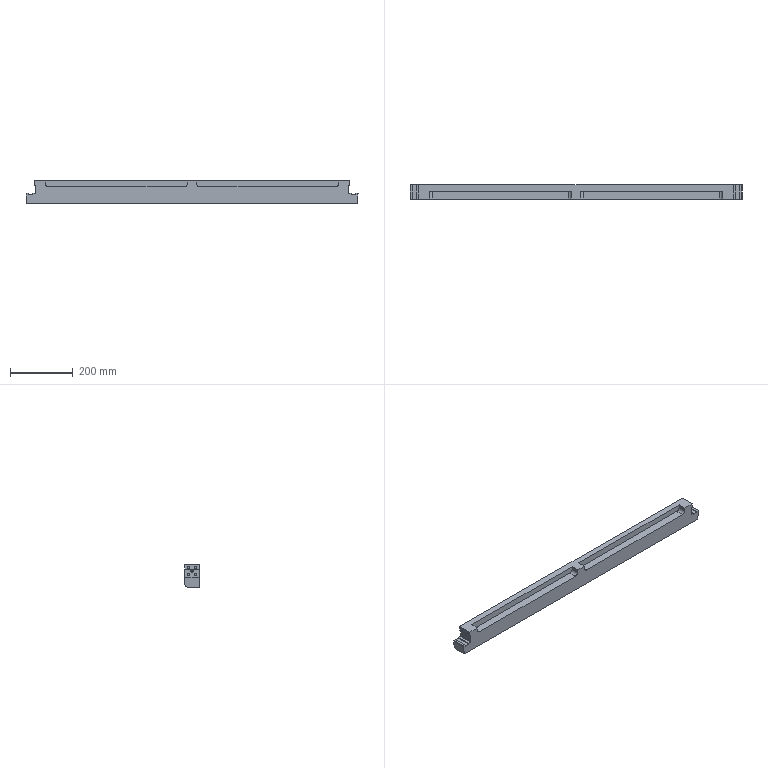NC program | NX | posted with a generic post | part box 1056 x 45 x 72.5 mm
Whole program:
N10 G17 G21 G94 G90
(ZLEVEL_PROFILE_2 , TOOL : D12)
N12 T20 M6
N14 G54
N16 G17 G0 G90 X-200.083 Y18.15 B0. C0. S7500 M3
N18 G43 Z30. H20
N20 Z1.5
N22 G94 G1 X-266. Z-1.955 F1001.
N24 X-482. F3000.
N26 G3 X-486.4 Y13.75 R4.4
N28 X-482. Y9.35 R4.4
N30 G1 X-50.
N32 G3 X-45.6 Y13.75 R4.4
N34 X-50. Y18.15 R4.4
N36 G1 X-266.
N38 X-377.976 Z-3.909
N40 X-482.
N42 G3 X-486.4 Y13.75 R4.4
N44 X-482. Y9.35 R4.4
N46 G1 X-50.
N48 G3 X-45.6 Y13.75 R4.4
N50 X-50. Y18.15 R4.4
N52 G1 X-266.
N54 X-377.976 Z-5.864
N56 X-482.
N58 G3 X-486.4 Y13.75 R4.4
N60 X-482. Y9.35 R4.4
N62 G1 X-50.
N64 G3 X-45.6 Y13.75 R4.4
N66 X-50. Y18.15 R4.4
N68 G1 X-266.
N70 X-377.976 Z-7.818
N72 X-482.
N74 G3 X-486.4 Y13.75 R4.4
N76 X-482. Y9.35 R4.4
N78 G1 X-50.
N80 G3 X-45.6 Y13.75 R4.4
N82 X-50. Y18.15 R4.4
N84 G1 X-266.
N86 X-377.976 Z-9.773
N88 X-482.
N90 G3 X-486.4 Y13.75 R4.4
N92 X-482. Y9.35 R4.4
N94 G1 X-50.
N96 G3 X-45.6 Y13.75 R4.4
N98 X-50. Y18.15 R4.4
N100 G1 X-266.
N102 X-377.976 Z-11.727
N104 X-482.
N106 G3 X-486.4 Y13.75 R4.4
N108 X-482. Y9.35 R4.4
N110 G1 X-50.
N112 G3 X-45.6 Y13.75 R4.4
N114 X-50. Y18.15 R4.4
N116 G1 X-266.
N118 X-377.976 Z-13.682
N120 X-482.
N122 G3 X-486.4 Y13.75 R4.4
N124 X-482. Y9.35 R4.4
N126 G1 X-50.
N128 G3 X-45.6 Y13.75 R4.4
N130 X-50. Y18.15 R4.4
N132 G1 X-266.
N134 X-377.976 Z-15.636
N136 X-482.
N138 G3 X-486.4 Y13.75 R4.4
N140 X-482. Y9.35 R4.4
N142 G1 X-50.
N144 G3 X-45.6 Y13.75 R4.4
N146 X-50. Y18.15 R4.4
N148 G1 X-266.
N150 X-377.976 Z-17.591
N152 X-482.
N154 G3 X-486.4 Y13.75 R4.4
N156 X-482. Y9.35 R4.4
N158 G1 X-50.
N160 G3 X-45.6 Y13.75 R4.4
N162 X-50. Y18.15 R4.4
N164 G1 X-266.
N166 X-377.976 Z-19.545
N168 X-482.
N170 G3 X-486.4 Y13.75 R4.4
N172 X-482. Y9.35 R4.4
N174 G1 X-50.
N176 G3 X-45.6 Y13.75 R4.4
N178 X-50. Y18.15 R4.4
N180 G1 X-266.
N182 X-377.976 Z-21.5
N184 X-482.
N186 G3 X-486.4 Y13.75 R4.4
N188 X-482. Y9.35 R4.4
N190 G1 X-50.
N192 G3 X-45.6 Y13.75 R4.4
N194 X-50. Y18.15 R4.4
N196 G1 X-377.976
N198 G3 X-379.015 Y17.55 R1.2
N200 G1 X-379.361 Y16.95
N202 Z-20.3
N204 G0 Z30.
N206 X331.917 Y18.15
N208 Z1.5
N210 G1 X266. Z-1.955 F1001.
N212 X50. F3000.
N214 G3 X45.6 Y13.75 R4.4
N216 X50. Y9.35 R4.4
N218 G1 X482.
N220 G3 X486.4 Y13.75 R4.4
N222 X482. Y18.15 R4.4
N224 G1 X266.
N226 X154.024 Z-3.909
N228 X50.
N230 G3 X45.6 Y13.75 R4.4
N232 X50. Y9.35 R4.4
N234 G1 X482.
N236 G3 X486.4 Y13.75 R4.4
N238 X482. Y18.15 R4.4
N240 G1 X266.
N242 X154.024 Z-5.864
N244 X50.
N246 G3 X45.6 Y13.75 R4.4
N248 X50. Y9.35 R4.4
N250 G1 X482.
N252 G3 X486.4 Y13.75 R4.4
N254 X482. Y18.15 R4.4
N256 G1 X266.
N258 X154.024 Z-7.818
N260 X50.
N262 G3 X45.6 Y13.75 R4.4
N264 X50. Y9.35 R4.4
N266 G1 X482.
N268 G3 X486.4 Y13.75 R4.4
N270 X482. Y18.15 R4.4
N272 G1 X266.
N274 X154.024 Z-9.773
N276 X50.
N278 G3 X45.6 Y13.75 R4.4
N280 X50. Y9.35 R4.4
N282 G1 X482.
N284 G3 X486.4 Y13.75 R4.4
N286 X482. Y18.15 R4.4
N288 G1 X266.
N290 X154.024 Z-11.727
N292 X50.
N294 G3 X45.6 Y13.75 R4.4
N296 X50. Y9.35 R4.4
N298 G1 X482.
N300 G3 X486.4 Y13.75 R4.4
N302 X482. Y18.15 R4.4
N304 G1 X266.
N306 X154.024 Z-13.682
N308 X50.
N310 G3 X45.6 Y13.75 R4.4
N312 X50. Y9.35 R4.4
N314 G1 X482.
N316 G3 X486.4 Y13.75 R4.4
N318 X482. Y18.15 R4.4
N320 G1 X266.
N322 X154.024 Z-15.636
N324 X50.
N326 G3 X45.6 Y13.75 R4.4
N328 X50. Y9.35 R4.4
N330 G1 X482.
N332 G3 X486.4 Y13.75 R4.4
N334 X482. Y18.15 R4.4
N336 G1 X266.
N338 X154.024 Z-17.591
N340 X50.
N342 G3 X45.6 Y13.75 R4.4
N344 X50. Y9.35 R4.4
N346 G1 X482.
N348 G3 X486.4 Y13.75 R4.4
N350 X482. Y18.15 R4.4
N352 G1 X266.
N354 X154.024 Z-19.545
N356 X50.
N358 G3 X45.6 Y13.75 R4.4
N360 X50. Y9.35 R4.4
N362 G1 X482.
N364 G3 X486.4 Y13.75 R4.4
N366 X482. Y18.15 R4.4
N368 G1 X266.
N370 X154.024 Z-21.5
N372 X50.
N374 G3 X45.6 Y13.75 R4.4
N376 X50. Y9.35 R4.4
N378 G1 X482.
N380 G3 X486.4 Y13.75 R4.4
N382 X482. Y18.15 R4.4
N384 G1 X154.024
N386 G3 X152.985 Y17.55 R1.2
N388 G1 X152.639 Y16.95
N390 Z-20.3
N392 G0 Z30.
(11 , TOOL : D12)
N394 X-49.459 Y15.779 S6500
N396 Z-20.5
N398 G1 Z-21.5 F1000.
N400 X-48.961 Y17.65
N402 G3 X-50. Y18.25 R1.2
N404 G1 X-482.
N406 G3 X-486.5 Y13.75 R4.5
N408 X-482. Y9.25 R4.5
N410 G1 X-50.
N412 G3 X-45.5 Y13.75 R4.5
N414 X-50. Y18.25 R4.5
N416 X-51.039 Y17.65 R1.2
N418 G1 X-52.078 Y15.85
N420 Z-20.5
N422 G0 Z30.
N424 X482.541 Y15.779
N426 Z-20.5
N428 G1 Z-21.5
N430 X483.039 Y17.65
N432 G3 X482. Y18.25 R1.2
N434 G1 X50.
N436 G3 X45.5 Y13.75 R4.5
N438 X50. Y9.25 R4.5
N440 G1 X482.
N442 G3 X486.5 Y13.75 R4.5
N444 X482. Y18.25 R4.5
N446 X480.961 Y17.65 R1.2
N448 G1 X479.922 Y15.85
N450 Z-20.5
N452 G0 Z30.
N454 M5
(ZLEVEL_PROFILE_1_COPY_1_COPY_COPY_1_COPY_1_COPY_1 , TOOL : D10A45)
N456 T07 M6
N458 G54
N460 G17 G0 G90 X-48.131 Y21.013 B0. C0. S7500 M3
N462 G43 Z30. H7
N464 Z-1.
N466 G94 G1 Z-2. F1000.
N468 X-49.134 Y22.75
N470 G3 X-50. Y23.25 R1.
N472 G1 X-482.
N474 G3 X-491.5 Y13.75 R9.5
N476 X-482. Y4.25 R9.5
N478 G1 X-50.
N480 G3 X-40.5 Y13.75 R9.5
N482 X-50. Y23.25 R9.5
N484 X-50.866 Y22.75 R1.
N486 G1 X-51.732 Y21.25
N488 Z-1.
N490 G0 Z30.
N492 X483.869 Y21.013
N494 Z-1.
N496 G1 Z-2.
N498 X482.866 Y22.75
N500 G3 X482. Y23.25 R1.
N502 G1 X50.
N504 G3 X40.5 Y13.75 R9.5
N506 X50. Y4.25 R9.5
N508 G1 X482.
N510 G3 X491.5 Y13.75 R9.5
N512 X482. Y23.25 R9.5
N514 X481.134 Y22.75 R1.
N516 G1 X480.268 Y21.25
N518 Z-1.
N520 G0 Z30.
(ZLEVEL_PROFILE_1_COPY_1_COPY_COPY_1_COPY_COPY_1 , TOOL : D10A45)
N522 X527.204 Y43.069 S7000
N524 Z-0.5
N526 G1 Z-1.5
N528 X526.123 Y42.145
N530 G3 X525.79 Y41.202 R1.
N532 G1 X525.82 Y41.04
N534 X529.287 Y6.378
N536 X529.293 Y6.247
N538 Y4.249
N540 G2 X528.915 Y3.336 R1.335
N542 G1 X528.414 Y2.835
N544 G2 X527.501 Y2.457 R1.291
N546 G1 X521.599
N548 G2 X520.307 Y3.749 R1.292
N550 G1 Y5.557
N552 X507.693
N554 Y3.749
N556 G2 X506.401 Y2.457 R1.292
N558 G1 X498.293
N560 Y-20.557
N562 X499.901
N564 G2 X501.193 Y-21.849 R1.292
N566 G1 Y-36.24
N568 Y-44.172
N570 G3 X501.693 Y-45.038 R1.
N572 G1 X502.85 Y-45.706
N574 Z-0.5
N576 G0 Z30.
N578 X-502.818 Y-45.768
N580 Z-0.5
N582 G1 Z-1.5
N584 X-501.689 Y-45.115
N586 G3 X-501.189 Y-44.249 R1.
N588 G1 X-501.193 Y-36.24
N590 Y-21.849
N592 G2 X-499.901 Y-20.557 R1.292
N594 G1 X-498.293
N596 Y2.457
N598 X-506.401
N600 G2 X-507.693 Y3.749 R1.292
N602 G1 Y5.557
N604 X-520.307
N606 Y3.749
N608 G2 X-521.599 Y2.457 R1.292
N610 G1 X-527.501
N612 G2 X-528.414 Y2.835 R1.291
N614 G1 X-528.915 Y3.336
N616 G2 X-529.293 Y4.249 R1.335
N618 G1 Y6.247
N620 X-529.287 Y6.378
N622 X-525.82 Y41.04
N624 X-525.79 Y41.202
N626 G3 X-526.123 Y42.145 R1.
N628 G1 X-527.204 Y43.069
N630 Z-0.5
N632 G0 Z30.
N634 M5
(PLANAR_PROFILE_COPY_COPY_COPY , TOOL : D30内R刀)
N636 T09 M6
N638 G54
N640 G17 G0 G90 X-532. Y47.25 B0. C0. S7500 M3
N642 G43 Z30. H9
N644 Z-7.
N646 G94 G1 Z-10. F1250.
N648 G3 X-526. Y44.25 R7.5
N650 G1 X526.
N652 G3 X532. Y47.25 R7.5
N654 G1 Z-7.
N656 G0 Z30.
(PLANAR_PROFILE_COPY_COPY_COPY_COPY , TOOL : D30内R刀)
N658 X-532. Y46.25
N660 Z-7.
N662 G1 Z-10.
N664 G3 X-526. Y43.25 R7.5
N666 G1 X526.
N668 G3 X532. Y46.25 R7.5
N670 G1 Z-7.
N672 G0 Z30.
(PLANAR_PROFILE_COPY_COPY_COPY_COPY_COPY , TOOL : D30内R刀)
N674 X-532. Y45.25
N676 Z-7.
N678 G1 Z-10.
N680 G3 X-526. Y42.25 R7.5
N682 G1 X526.
N684 G3 X532. Y45.25 R7.5
N686 G1 Z-7.
N688 G0 Z30.
(PLANAR_PROFILE_COPY_COPY_COPY_COPY_COPY_COPY , TOOL : D30内R刀)
N690 X-532. Y44.25
N692 Z-7.
N694 G1 Z-10.
N696 G3 X-526. Y41.25 R7.5
N698 G1 X526.
N700 G3 X532. Y44.25 R7.5
N702 G1 Z-7.
N704 G0 Z30.
N706 M5
N708 M2